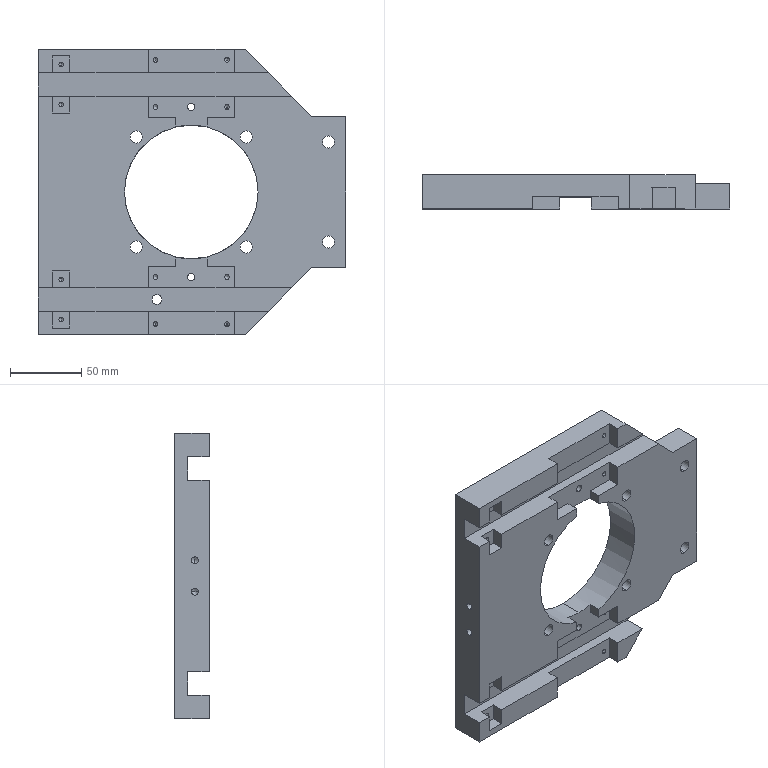Part | SolidWorks | features BaseBody 1 | 1 solid | 135 faces | box 215 x 24 x 200 mm | volume 612266 mm3 | plane 59 | cylinder 48 | cone 28 | commonest cylinder face diameters 3.3 x24 8.5 x12 5 x8 6.8 x2 93.5 x2